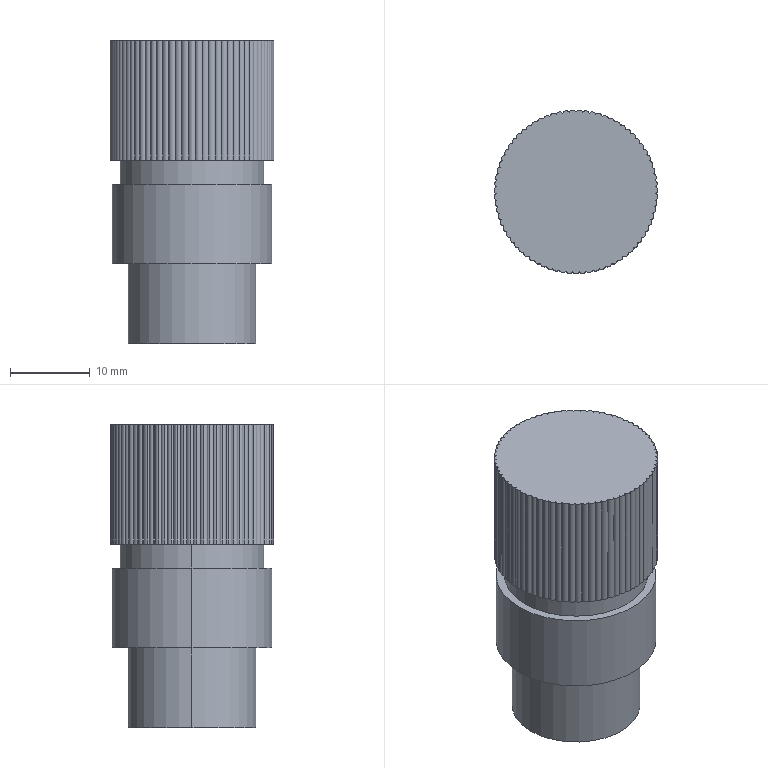Part | STEP file | Black terminal post | 1 solid | 186 faces | box 20.458 x 20.454 x 38 mm | volume 10782 mm3 | cylinder 181 | plane 5 | commonest cylinder face diameters 0.964 x100 20 x77 16 x2 18 x2